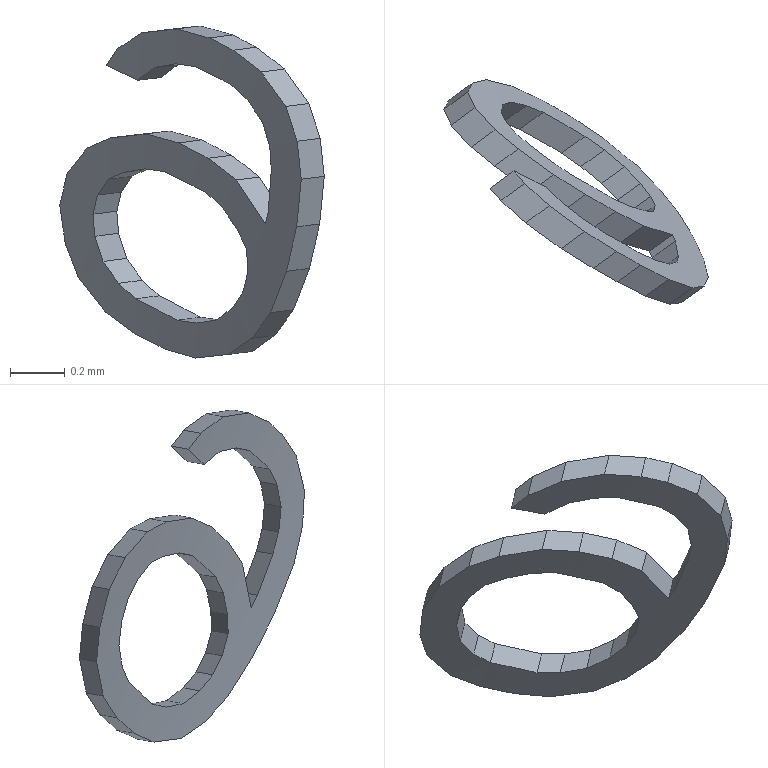Part | SolidWorks | features BaseBody 1 | 1 solid | 62 faces | box 0.9706 x 0.8253 x 1.218 mm | volume 0.04974 mm3 | plane 60 | cylinder 2 | commonest cylinder face diameters 16.8 x1 17 x1